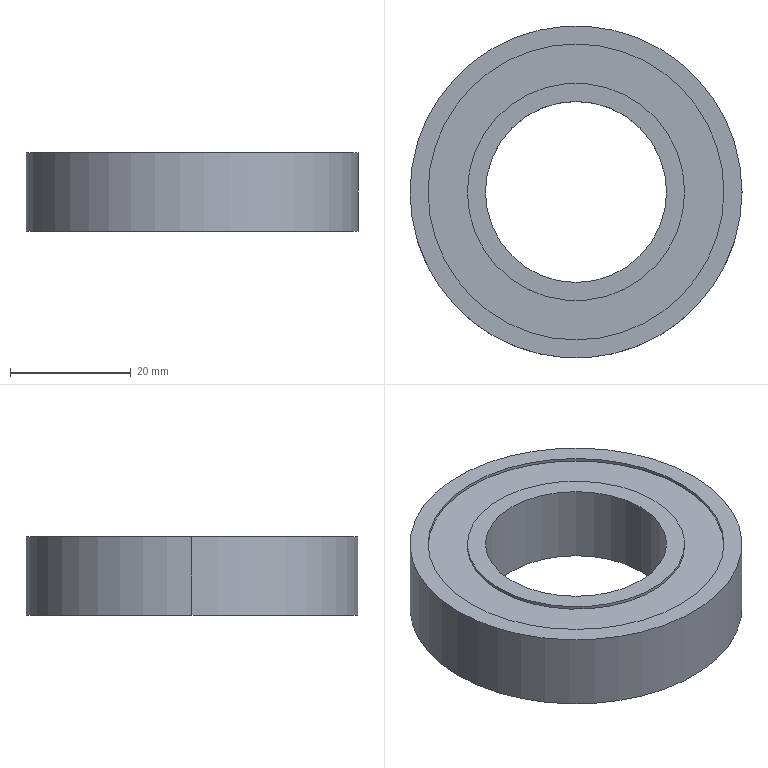Part | SolidWorks | features Extrusion 1, ICE 1, MirrorPattern 1 | 1 solid | 18 faces | box 55 x 55 x 13 mm | volume 20829 mm3 | cylinder 12 | plane 6 | commonest cylinder face diameters 36 x4 49 x4 30 x2 55 x2
STEP:
#1=CARTESIAN_POINT('',(18.,0.,-6.));
#2=VERTEX_POINT('',#1);
#3=CARTESIAN_POINT('',(-18.,0.,-6.));
#4=VERTEX_POINT('',#3);
#5=CARTESIAN_POINT('',(0.,0.,-6.));
#6=DIRECTION('',(0.,0.,1.));
#7=DIRECTION('',(1.,0.,0.));
#8=AXIS2_PLACEMENT_3D('',#5,#6,#7);
#9=CIRCLE('',#8,18.);
#10=EDGE_CURVE('',#2,#4,#9,.T.);
#11=ORIENTED_EDGE('',*,*,#10,.F.);
#12=CARTESIAN_POINT('',(18.,0.,-6.5));
#13=VERTEX_POINT('',#12);
#14=CARTESIAN_POINT('',(18.,0.,-6.));
#15=DIRECTION('',(0.,0.,-1.));
#16=VECTOR('',#15,1000.);
#17=LINE('',#14,#16);
#18=EDGE_CURVE('',#2,#13,#17,.T.);
#19=ORIENTED_EDGE('',*,*,#18,.T.);
#20=CARTESIAN_POINT('',(-18.,0.,-6.5));
#21=VERTEX_POINT('',#20);
#22=CARTESIAN_POINT('',(0.,0.,-6.5));
#23=DIRECTION('',(0.,0.,1.));
#24=DIRECTION('',(1.,0.,0.));
#25=AXIS2_PLACEMENT_3D('',#22,#23,#24);
#26=CIRCLE('',#25,18.);
#27=EDGE_CURVE('',#13,#21,#26,.T.);
#28=ORIENTED_EDGE('',*,*,#27,.T.);
#29=CARTESIAN_POINT('',(-18.,0.,-6.));
#30=DIRECTION('',(0.,0.,-1.));
#31=VECTOR('',#30,1000.);
#32=LINE('',#29,#31);
#33=EDGE_CURVE('',#4,#21,#32,.T.);
#34=ORIENTED_EDGE('',*,*,#33,.F.);
#35=EDGE_LOOP('',(#11,#19,#28,#34));
#36=FACE_OUTER_BOUND('',#35,.T.);
#37=CARTESIAN_POINT('',(0.,0.,-6.));
#38=DIRECTION('',(0.,0.,-1.));
#39=DIRECTION('',(-1.,0.,0.));
#40=AXIS2_PLACEMENT_3D('',#37,#38,#39);
#41=CYLINDRICAL_SURFACE('',#40,18.);
#42=ADVANCED_FACE('',(#36),#41,.T.);
#43=CARTESIAN_POINT('',(-24.5,0.,-6.));
#44=VERTEX_POINT('',#43);
#45=CARTESIAN_POINT('',(24.5,0.,-6.));
#46=VERTEX_POINT('',#45);
#47=CARTESIAN_POINT('',(0.,0.,-6.));
#48=DIRECTION('',(0.,0.,1.));
#49=DIRECTION('',(1.,0.,0.));
#50=AXIS2_PLACEMENT_3D('',#47,#48,#49);
#51=CIRCLE('',#50,24.5);
#52=EDGE_CURVE('',#44,#46,#51,.T.);
#53=ORIENTED_EDGE('',*,*,#52,.T.);
#54=CARTESIAN_POINT('',(24.5,0.,-6.5));
#55=VERTEX_POINT('',#54);
#56=CARTESIAN_POINT('',(24.5,0.,-6.));
#57=DIRECTION('',(0.,0.,-1.));
#58=VECTOR('',#57,1000.);
#59=LINE('',#56,#58);
#60=EDGE_CURVE('',#46,#55,#59,.T.);
#61=ORIENTED_EDGE('',*,*,#60,.T.);
#62=CARTESIAN_POINT('',(-24.5,0.,-6.5));
#63=VERTEX_POINT('',#62);
#64=CARTESIAN_POINT('',(0.,0.,-6.5));
#65=DIRECTION('',(0.,0.,1.));
#66=DIRECTION('',(1.,0.,0.));
#67=AXIS2_PLACEMENT_3D('',#64,#65,#66);
#68=CIRCLE('',#67,24.5);
#69=EDGE_CURVE('',#63,#55,#68,.T.);
#70=ORIENTED_EDGE('',*,*,#69,.F.);
#71=CARTESIAN_POINT('',(-24.5,0.,-6.));
#72=DIRECTION('',(0.,0.,-1.));
#73=VECTOR('',#72,1000.);
#74=LINE('',#71,#73);
#75=EDGE_CURVE('',#44,#63,#74,.T.);
#76=ORIENTED_EDGE('',*,*,#75,.F.);
#77=EDGE_LOOP('',(#53,#61,#70,#76));
#78=FACE_OUTER_BOUND('',#77,.T.);
#79=CARTESIAN_POINT('',(0.,0.,-6.));
#80=DIRECTION('',(0.,0.,-1.));
#81=DIRECTION('',(-1.,0.,0.));
#82=AXIS2_PLACEMENT_3D('',#79,#80,#81);
#83=CYLINDRICAL_SURFACE('',#82,24.5);
#84=ADVANCED_FACE('',(#78),#83,.F.);
#85=CARTESIAN_POINT('',(18.,0.,6.));
#86=VERTEX_POINT('',#85);
#87=CARTESIAN_POINT('',(-18.,0.,6.));
#88=VERTEX_POINT('',#87);
#89=CARTESIAN_POINT('',(0.,0.,6.));
#90=DIRECTION('',(0.,0.,1.));
#91=DIRECTION('',(1.,0.,0.));
#92=AXIS2_PLACEMENT_3D('',#89,#90,#91);
#93=CIRCLE('',#92,18.);
#94=EDGE_CURVE('',#86,#88,#93,.T.);
#95=ORIENTED_EDGE('',*,*,#94,.T.);
#96=CARTESIAN_POINT('',(-18.,0.,6.5));
#97=VERTEX_POINT('',#96);
#98=CARTESIAN_POINT('',(-18.,0.,6.));
#99=DIRECTION('',(0.,0.,1.));
#100=VECTOR('',#99,1000.);
#101=LINE('',#98,#100);
#102=EDGE_CURVE('',#88,#97,#101,.T.);
#103=ORIENTED_EDGE('',*,*,#102,.T.);
#104=CARTESIAN_POINT('',(18.,0.,6.5));
#105=VERTEX_POINT('',#104);
#106=CARTESIAN_POINT('',(0.,0.,6.5));
#107=DIRECTION('',(0.,0.,1.));
#108=DIRECTION('',(1.,0.,0.));
#109=AXIS2_PLACEMENT_3D('',#106,#107,#108);
#110=CIRCLE('',#109,18.);
#111=EDGE_CURVE('',#105,#97,#110,.T.);
#112=ORIENTED_EDGE('',*,*,#111,.F.);
#113=CARTESIAN_POINT('',(18.,0.,6.));
#114=DIRECTION('',(0.,0.,1.));
#115=VECTOR('',#114,1000.);
#116=LINE('',#113,#115);
#117=EDGE_CURVE('',#86,#105,#116,.T.);
#118=ORIENTED_EDGE('',*,*,#117,.F.);
#119=EDGE_LOOP('',(#95,#103,#112,#118));
#120=FACE_OUTER_BOUND('',#119,.T.);
#121=CARTESIAN_POINT('',(0.,0.,6.));
#122=DIRECTION('',(0.,0.,1.));
#123=DIRECTION('',(1.,0.,0.));
#124=AXIS2_PLACEMENT_3D('',#121,#122,#123);
#125=CYLINDRICAL_SURFACE('',#124,18.);
#126=ADVANCED_FACE('',(#120),#125,.T.);
#127=CARTESIAN_POINT('',(-24.5,0.,6.));
#128=VERTEX_POINT('',#127);
#129=CARTESIAN_POINT('',(24.5,0.,6.));
#130=VERTEX_POINT('',#129);
#131=CARTESIAN_POINT('',(0.,0.,6.));
#132=DIRECTION('',(0.,0.,1.));
#133=DIRECTION('',(1.,0.,0.));
#134=AXIS2_PLACEMENT_3D('',#131,#132,#133);
#135=CIRCLE('',#134,24.5);
#136=EDGE_CURVE('',#128,#130,#135,.T.);
#137=ORIENTED_EDGE('',*,*,#136,.F.);
#138=CARTESIAN_POINT('',(-24.5,0.,6.5));
#139=VERTEX_POINT('',#138);
#140=CARTESIAN_POINT('',(-24.5,0.,6.));
#141=DIRECTION('',(0.,0.,1.));
#142=VECTOR('',#141,1000.);
#143=LINE('',#140,#142);
#144=EDGE_CURVE('',#128,#139,#143,.T.);
#145=ORIENTED_EDGE('',*,*,#144,.T.);
#146=CARTESIAN_POINT('',(24.5,0.,6.5));
#147=VERTEX_POINT('',#146);
#148=CARTESIAN_POINT('',(0.,0.,6.5));
#149=DIRECTION('',(0.,0.,1.));
#150=DIRECTION('',(1.,0.,0.));
#151=AXIS2_PLACEMENT_3D('',#148,#149,#150);
#152=CIRCLE('',#151,24.5);
#153=EDGE_CURVE('',#139,#147,#152,.T.);
#154=ORIENTED_EDGE('',*,*,#153,.T.);
#155=CARTESIAN_POINT('',(24.5,0.,6.));
#156=DIRECTION('',(0.,0.,1.));
#157=VECTOR('',#156,1000.);
#158=LINE('',#155,#157);
#159=EDGE_CURVE('',#130,#147,#158,.T.);
#160=ORIENTED_EDGE('',*,*,#159,.F.);
#161=EDGE_LOOP('',(#137,#145,#154,#160));
#162=FACE_OUTER_BOUND('',#161,.T.);
#163=CARTESIAN_POINT('',(0.,0.,6.));
#164=DIRECTION('',(0.,0.,1.));
#165=DIRECTION('',(1.,0.,0.));
#166=AXIS2_PLACEMENT_3D('',#163,#164,#165);
#167=CYLINDRICAL_SURFACE('',#166,24.5);
#168=ADVANCED_FACE('',(#162),#167,.F.);
#169=CARTESIAN_POINT('',(-15.,0.,6.5));
#170=VERTEX_POINT('',#169);
#171=CARTESIAN_POINT('',(15.,0.,6.5));
#172=VERTEX_POINT('',#171);
#173=CARTESIAN_POINT('',(0.,0.,6.5));
#174=DIRECTION('',(0.,0.,1.));
#175=DIRECTION('',(1.,0.,0.));
#176=AXIS2_PLACEMENT_3D('',#173,#174,#175);
#177=CIRCLE('',#176,15.);
#178=EDGE_CURVE('',#170,#172,#177,.T.);
#179=ORIENTED_EDGE('',*,*,#178,.T.);
#180=CARTESIAN_POINT('',(15.,0.,-6.5));
#181=VERTEX_POINT('',#180);
#182=CARTESIAN_POINT('',(15.,0.,6.5));
#183=DIRECTION('',(0.,0.,-1.));
#184=VECTOR('',#183,1000.);
#185=LINE('',#182,#184);
#186=EDGE_CURVE('',#172,#181,#185,.T.);
#187=ORIENTED_EDGE('',*,*,#186,.T.);
#188=CARTESIAN_POINT('',(-15.,0.,-6.5));
#189=VERTEX_POINT('',#188);
#190=CARTESIAN_POINT('',(0.,0.,-6.5));
#191=DIRECTION('',(0.,0.,1.));
#192=DIRECTION('',(1.,0.,0.));
#193=AXIS2_PLACEMENT_3D('',#190,#191,#192);
#194=CIRCLE('',#193,15.);
#195=EDGE_CURVE('',#189,#181,#194,.T.);
#196=ORIENTED_EDGE('',*,*,#195,.F.);
#197=CARTESIAN_POINT('',(-15.,0.,6.5));
#198=DIRECTION('',(0.,0.,-1.));
#199=VECTOR('',#198,1000.);
#200=LINE('',#197,#199);
#201=EDGE_CURVE('',#170,#189,#200,.T.);
#202=ORIENTED_EDGE('',*,*,#201,.F.);
#203=EDGE_LOOP('',(#179,#187,#196,#202));
#204=FACE_OUTER_BOUND('',#203,.T.);
#205=CARTESIAN_POINT('',(0.,0.,6.5));
#206=DIRECTION('',(0.,0.,-1.));
#207=DIRECTION('',(-1.,0.,0.));
#208=AXIS2_PLACEMENT_3D('',#205,#206,#207);
#209=CYLINDRICAL_SURFACE('',#208,15.);
#210=ADVANCED_FACE('',(#204),#209,.F.);
#211=CARTESIAN_POINT('',(27.5,0.,6.5));
#212=VERTEX_POINT('',#211);
#213=CARTESIAN_POINT('',(-27.5,0.,6.5));
#214=VERTEX_POINT('',#213);
#215=CARTESIAN_POINT('',(0.,0.,6.5));
#216=DIRECTION('',(0.,0.,1.));
#217=DIRECTION('',(1.,0.,0.));
#218=AXIS2_PLACEMENT_3D('',#215,#216,#217);
#219=CIRCLE('',#218,27.5);
#220=EDGE_CURVE('',#212,#214,#219,.T.);
#221=ORIENTED_EDGE('',*,*,#220,.F.);
#222=CARTESIAN_POINT('',(27.5,0.,-6.5));
#223=VERTEX_POINT('',#222);
#224=CARTESIAN_POINT('',(27.5,0.,6.5));
#225=DIRECTION('',(0.,0.,-1.));
#226=VECTOR('',#225,1000.);
#227=LINE('',#224,#226);
#228=EDGE_CURVE('',#212,#223,#227,.T.);
#229=ORIENTED_EDGE('',*,*,#228,.T.);
#230=CARTESIAN_POINT('',(-27.5,0.,-6.5));
#231=VERTEX_POINT('',#230);
#232=CARTESIAN_POINT('',(0.,0.,-6.5));
#233=DIRECTION('',(0.,0.,1.));
#234=DIRECTION('',(1.,0.,0.));
#235=AXIS2_PLACEMENT_3D('',#232,#233,#234);
#236=CIRCLE('',#235,27.5);
#237=EDGE_CURVE('',#223,#231,#236,.T.);
#238=ORIENTED_EDGE('',*,*,#237,.T.);
#239=CARTESIAN_POINT('',(-27.5,0.,6.5));
#240=DIRECTION('',(0.,0.,-1.));
#241=VECTOR('',#240,1000.);
#242=LINE('',#239,#241);
#243=EDGE_CURVE('',#214,#231,#242,.T.);
#244=ORIENTED_EDGE('',*,*,#243,.F.);
#245=EDGE_LOOP('',(#221,#229,#238,#244));
#246=FACE_OUTER_BOUND('',#245,.T.);
#247=CARTESIAN_POINT('',(0.,0.,6.5));
#248=DIRECTION('',(0.,0.,-1.));
#249=DIRECTION('',(-1.,0.,0.));
#250=AXIS2_PLACEMENT_3D('',#247,#248,#249);
#251=CYLINDRICAL_SURFACE('',#250,27.5);
#252=ADVANCED_FACE('',(#246),#251,.T.);
#253=CARTESIAN_POINT('',(0.,0.,-6.5));
#254=DIRECTION('',(0.,0.,1.));
#255=DIRECTION('',(1.,0.,0.));
#256=AXIS2_PLACEMENT_3D('',#253,#254,#255);
#257=CIRCLE('',#256,27.5);
#258=EDGE_CURVE('',#231,#223,#257,.T.);
#259=ORIENTED_EDGE('',*,*,#258,.F.);
#260=ORIENTED_EDGE('',*,*,#237,.F.);
#261=EDGE_LOOP('',(#259,#260));
#262=FACE_OUTER_BOUND('',#261,.T.);
#263=ORIENTED_EDGE('',*,*,#69,.T.);
#264=CARTESIAN_POINT('',(0.,0.,-6.5));
#265=DIRECTION('',(0.,0.,1.));
#266=DIRECTION('',(1.,0.,0.));
#267=AXIS2_PLACEMENT_3D('',#264,#265,#266);
#268=CIRCLE('',#267,24.5);
#269=EDGE_CURVE('',#55,#63,#268,.T.);
#270=ORIENTED_EDGE('',*,*,#269,.T.);
#271=EDGE_LOOP('',(#263,#270));
#272=FACE_BOUND('',#271,.T.);
#273=CARTESIAN_POINT('',(0.,0.,-6.5));
#274=DIRECTION('',(0.,0.,1.));
#275=DIRECTION('',(1.,0.,0.));
#276=AXIS2_PLACEMENT_3D('',#273,#274,#275);
#277=PLANE('',#276);
#278=ADVANCED_FACE('',(#262,#272),#277,.F.);
#279=ORIENTED_EDGE('',*,*,#178,.F.);
#280=CARTESIAN_POINT('',(0.,0.,6.5));
#281=DIRECTION('',(0.,0.,1.));
#282=DIRECTION('',(1.,0.,0.));
#283=AXIS2_PLACEMENT_3D('',#280,#281,#282);
#284=CIRCLE('',#283,15.);
#285=EDGE_CURVE('',#172,#170,#284,.T.);
#286=ORIENTED_EDGE('',*,*,#285,.F.);
#287=EDGE_LOOP('',(#279,#286));
#288=FACE_BOUND('',#287,.T.);
#289=ORIENTED_EDGE('',*,*,#111,.T.);
#290=CARTESIAN_POINT('',(0.,0.,6.5));
#291=DIRECTION('',(0.,0.,1.));
#292=DIRECTION('',(1.,0.,0.));
#293=AXIS2_PLACEMENT_3D('',#290,#291,#292);
#294=CIRCLE('',#293,18.);
#295=EDGE_CURVE('',#97,#105,#294,.T.);
#296=ORIENTED_EDGE('',*,*,#295,.T.);
#297=EDGE_LOOP('',(#289,#296));
#298=FACE_OUTER_BOUND('',#297,.T.);
#299=CARTESIAN_POINT('',(0.,0.,6.5));
#300=DIRECTION('',(0.,0.,1.));
#301=DIRECTION('',(1.,0.,0.));
#302=AXIS2_PLACEMENT_3D('',#299,#300,#301);
#303=PLANE('',#302);
#304=ADVANCED_FACE('',(#288,#298),#303,.T.);
#305=CARTESIAN_POINT('',(0.,0.,6.5));
#306=DIRECTION('',(0.,0.,1.));
#307=DIRECTION('',(1.,0.,0.));
#308=AXIS2_PLACEMENT_3D('',#305,#306,#307);
#309=CIRCLE('',#308,24.5);
#310=EDGE_CURVE('',#147,#139,#309,.T.);
#311=ORIENTED_EDGE('',*,*,#310,.F.);
#312=ORIENTED_EDGE('',*,*,#153,.F.);
#313=EDGE_LOOP('',(#311,#312));
#314=FACE_BOUND('',#313,.T.);
#315=CARTESIAN_POINT('',(0.,0.,6.5));
#316=DIRECTION('',(0.,0.,1.));
#317=DIRECTION('',(1.,0.,0.));
#318=AXIS2_PLACEMENT_3D('',#315,#316,#317);
#319=CIRCLE('',#318,27.5);
#320=EDGE_CURVE('',#214,#212,#319,.T.);
#321=ORIENTED_EDGE('',*,*,#320,.T.);
#322=ORIENTED_EDGE('',*,*,#220,.T.);
#323=EDGE_LOOP('',(#321,#322));
#324=FACE_OUTER_BOUND('',#323,.T.);
#325=CARTESIAN_POINT('',(0.,0.,6.5));
#326=DIRECTION('',(0.,0.,1.));
#327=DIRECTION('',(1.,0.,0.));
#328=AXIS2_PLACEMENT_3D('',#325,#326,#327);
#329=PLANE('',#328);
#330=ADVANCED_FACE('',(#314,#324),#329,.T.);
#331=CARTESIAN_POINT('',(0.,0.,-6.5));
#332=DIRECTION('',(0.,0.,1.));
#333=DIRECTION('',(1.,0.,0.));
#334=AXIS2_PLACEMENT_3D('',#331,#332,#333);
#335=CIRCLE('',#334,18.);
#336=EDGE_CURVE('',#21,#13,#335,.T.);
#337=ORIENTED_EDGE('',*,*,#336,.F.);
#338=ORIENTED_EDGE('',*,*,#27,.F.);
#339=EDGE_LOOP('',(#337,#338));
#340=FACE_OUTER_BOUND('',#339,.T.);
#341=ORIENTED_EDGE('',*,*,#195,.T.);
#342=CARTESIAN_POINT('',(0.,0.,-6.5));
#343=DIRECTION('',(0.,0.,1.));
#344=DIRECTION('',(1.,0.,0.));
#345=AXIS2_PLACEMENT_3D('',#342,#343,#344);
#346=CIRCLE('',#345,15.);
#347=EDGE_CURVE('',#181,#189,#346,.T.);
#348=ORIENTED_EDGE('',*,*,#347,.T.);
#349=EDGE_LOOP('',(#341,#348));
#350=FACE_BOUND('',#349,.T.);
#351=CARTESIAN_POINT('',(0.,0.,-6.5));
#352=DIRECTION('',(0.,0.,1.));
#353=DIRECTION('',(1.,0.,0.));
#354=AXIS2_PLACEMENT_3D('',#351,#352,#353);
#355=PLANE('',#354);
#356=ADVANCED_FACE('',(#340,#350),#355,.F.);
#357=ORIENTED_EDGE('',*,*,#228,.F.);
#358=ORIENTED_EDGE('',*,*,#320,.F.);
#359=ORIENTED_EDGE('',*,*,#243,.T.);
#360=ORIENTED_EDGE('',*,*,#258,.T.);
#361=EDGE_LOOP('',(#357,#358,#359,#360));
#362=FACE_OUTER_BOUND('',#361,.T.);
#363=CARTESIAN_POINT('',(0.,0.,6.5));
#364=DIRECTION('',(0.,0.,-1.));
#365=DIRECTION('',(-1.,0.,0.));
#366=AXIS2_PLACEMENT_3D('',#363,#364,#365);
#367=CYLINDRICAL_SURFACE('',#366,27.5);
#368=ADVANCED_FACE('',(#362),#367,.T.);
#369=ORIENTED_EDGE('',*,*,#186,.F.);
#370=ORIENTED_EDGE('',*,*,#285,.T.);
#371=ORIENTED_EDGE('',*,*,#201,.T.);
#372=ORIENTED_EDGE('',*,*,#347,.F.);
#373=EDGE_LOOP('',(#369,#370,#371,#372));
#374=FACE_OUTER_BOUND('',#373,.T.);
#375=CARTESIAN_POINT('',(0.,0.,6.5));
#376=DIRECTION('',(0.,0.,-1.));
#377=DIRECTION('',(-1.,0.,0.));
#378=AXIS2_PLACEMENT_3D('',#375,#376,#377);
#379=CYLINDRICAL_SURFACE('',#378,15.);
#380=ADVANCED_FACE('',(#374),#379,.F.);
#381=ORIENTED_EDGE('',*,*,#144,.F.);
#382=CARTESIAN_POINT('',(0.,0.,6.));
#383=DIRECTION('',(0.,0.,1.));
#384=DIRECTION('',(1.,0.,0.));
#385=AXIS2_PLACEMENT_3D('',#382,#383,#384);
#386=CIRCLE('',#385,24.5);
#387=EDGE_CURVE('',#130,#128,#386,.T.);
#388=ORIENTED_EDGE('',*,*,#387,.F.);
#389=ORIENTED_EDGE('',*,*,#159,.T.);
#390=ORIENTED_EDGE('',*,*,#310,.T.);
#391=EDGE_LOOP('',(#381,#388,#389,#390));
#392=FACE_OUTER_BOUND('',#391,.T.);
#393=CARTESIAN_POINT('',(0.,0.,6.));
#394=DIRECTION('',(0.,0.,1.));
#395=DIRECTION('',(1.,0.,0.));
#396=AXIS2_PLACEMENT_3D('',#393,#394,#395);
#397=CYLINDRICAL_SURFACE('',#396,24.5);
#398=ADVANCED_FACE('',(#392),#397,.F.);
#399=ORIENTED_EDGE('',*,*,#94,.F.);
#400=CARTESIAN_POINT('',(0.,0.,6.));
#401=DIRECTION('',(0.,0.,1.));
#402=DIRECTION('',(1.,0.,0.));
#403=AXIS2_PLACEMENT_3D('',#400,#401,#402);
#404=CIRCLE('',#403,18.);
#405=EDGE_CURVE('',#88,#86,#404,.T.);
#406=ORIENTED_EDGE('',*,*,#405,.F.);
#407=EDGE_LOOP('',(#399,#406));
#408=FACE_BOUND('',#407,.T.);
#409=ORIENTED_EDGE('',*,*,#387,.T.);
#410=ORIENTED_EDGE('',*,*,#136,.T.);
#411=EDGE_LOOP('',(#409,#410));
#412=FACE_OUTER_BOUND('',#411,.T.);
#413=CARTESIAN_POINT('',(0.,0.,6.));
#414=DIRECTION('',(0.,0.,1.));
#415=DIRECTION('',(1.,0.,0.));
#416=AXIS2_PLACEMENT_3D('',#413,#414,#415);
#417=PLANE('',#416);
#418=ADVANCED_FACE('',(#408,#412),#417,.T.);
#419=ORIENTED_EDGE('',*,*,#102,.F.);
#420=ORIENTED_EDGE('',*,*,#405,.T.);
#421=ORIENTED_EDGE('',*,*,#117,.T.);
#422=ORIENTED_EDGE('',*,*,#295,.F.);
#423=EDGE_LOOP('',(#419,#420,#421,#422));
#424=FACE_OUTER_BOUND('',#423,.T.);
#425=CARTESIAN_POINT('',(0.,0.,6.));
#426=DIRECTION('',(0.,0.,1.));
#427=DIRECTION('',(1.,0.,0.));
#428=AXIS2_PLACEMENT_3D('',#425,#426,#427);
#429=CYLINDRICAL_SURFACE('',#428,18.);
#430=ADVANCED_FACE('',(#424),#429,.T.);
#431=ORIENTED_EDGE('',*,*,#52,.F.);
#432=CARTESIAN_POINT('',(0.,0.,-6.));
#433=DIRECTION('',(0.,0.,1.));
#434=DIRECTION('',(1.,0.,0.));
#435=AXIS2_PLACEMENT_3D('',#432,#433,#434);
#436=CIRCLE('',#435,24.5);
#437=EDGE_CURVE('',#46,#44,#436,.T.);
#438=ORIENTED_EDGE('',*,*,#437,.F.);
#439=EDGE_LOOP('',(#431,#438));
#440=FACE_OUTER_BOUND('',#439,.T.);
#441=CARTESIAN_POINT('',(0.,0.,-6.));
#442=DIRECTION('',(0.,0.,1.));
#443=DIRECTION('',(1.,0.,0.));
#444=AXIS2_PLACEMENT_3D('',#441,#442,#443);
#445=CIRCLE('',#444,18.);
#446=EDGE_CURVE('',#4,#2,#445,.T.);
#447=ORIENTED_EDGE('',*,*,#446,.T.);
#448=ORIENTED_EDGE('',*,*,#10,.T.);
#449=EDGE_LOOP('',(#447,#448));
#450=FACE_BOUND('',#449,.T.);
#451=CARTESIAN_POINT('',(0.,0.,-6.));
#452=DIRECTION('',(0.,0.,-1.));
#453=DIRECTION('',(1.,0.,0.));
#454=AXIS2_PLACEMENT_3D('',#451,#452,#453);
#455=PLANE('',#454);
#456=ADVANCED_FACE('',(#440,#450),#455,.T.);
#457=ORIENTED_EDGE('',*,*,#60,.F.);
#458=ORIENTED_EDGE('',*,*,#437,.T.);
#459=ORIENTED_EDGE('',*,*,#75,.T.);
#460=ORIENTED_EDGE('',*,*,#269,.F.);
#461=EDGE_LOOP('',(#457,#458,#459,#460));
#462=FACE_OUTER_BOUND('',#461,.T.);
#463=CARTESIAN_POINT('',(0.,0.,-6.));
#464=DIRECTION('',(0.,0.,-1.));
#465=DIRECTION('',(-1.,0.,0.));
#466=AXIS2_PLACEMENT_3D('',#463,#464,#465);
#467=CYLINDRICAL_SURFACE('',#466,24.5);
#468=ADVANCED_FACE('',(#462),#467,.F.);
#469=ORIENTED_EDGE('',*,*,#18,.F.);
#470=ORIENTED_EDGE('',*,*,#446,.F.);
#471=ORIENTED_EDGE('',*,*,#33,.T.);
#472=ORIENTED_EDGE('',*,*,#336,.T.);
#473=EDGE_LOOP('',(#469,#470,#471,#472));
#474=FACE_OUTER_BOUND('',#473,.T.);
#475=CARTESIAN_POINT('',(0.,0.,-6.));
#476=DIRECTION('',(0.,0.,-1.));
#477=DIRECTION('',(-1.,0.,0.));
#478=AXIS2_PLACEMENT_3D('',#475,#476,#477);
#479=CYLINDRICAL_SURFACE('',#478,18.);
#480=ADVANCED_FACE('',(#474),#479,.T.);
#481=CLOSED_SHELL('',(#42,#84,#126,#168,#210,#252,#278,#304,#330,#356,#368,#380,#398,#418,#430,#456,#468,#480));
#482=MANIFOLD_SOLID_BREP('',#481);
#483=CARTESIAN_POINT('',(0.,0.,0.));
#484=DIRECTION('',(0.,0.,1.));
#485=DIRECTION('',(1.,0.,0.));
#486=AXIS2_PLACEMENT_3D('',#483,#484,#485);
#487=(LENGTH_UNIT()NAMED_UNIT(*)SI_UNIT(.MILLI.,.METRE.));
#488=UNCERTAINTY_MEASURE_WITH_UNIT(LENGTH_MEASURE(0.00001),#487,'','');
#489=(NAMED_UNIT(*)PLANE_ANGLE_UNIT()SI_UNIT($,.RADIAN.));
#490=(NAMED_UNIT(*)SI_UNIT($,.STERADIAN.)SOLID_ANGLE_UNIT());
#491=(GEOMETRIC_REPRESENTATION_CONTEXT(3)GLOBAL_UNCERTAINTY_ASSIGNED_CONTEXT((#488))GLOBAL_UNIT_ASSIGNED_CONTEXT((#487,#489,#490))REPRESENTATION_CONTEXT('',''));
#492=ADVANCED_BREP_SHAPE_REPRESENTATION('',(#482,#486),#491);